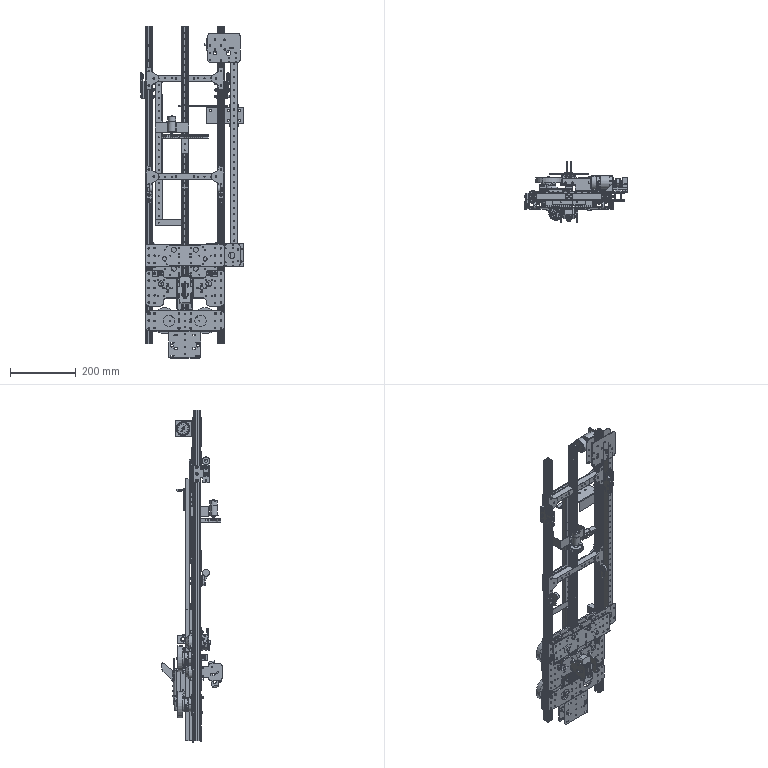Part | SolidWorks | features CompositeCurve 1 | 292 solids | 9504 faces | volume 2850499 mm3 | cylinder 4883 | plane 3675 | cone 617 | spline 321 | sphere 8 | commonest cylinder face diameters 3 x810 4.2 x490 5 x396 3.2 x288 3.5 x285 5.2 x272